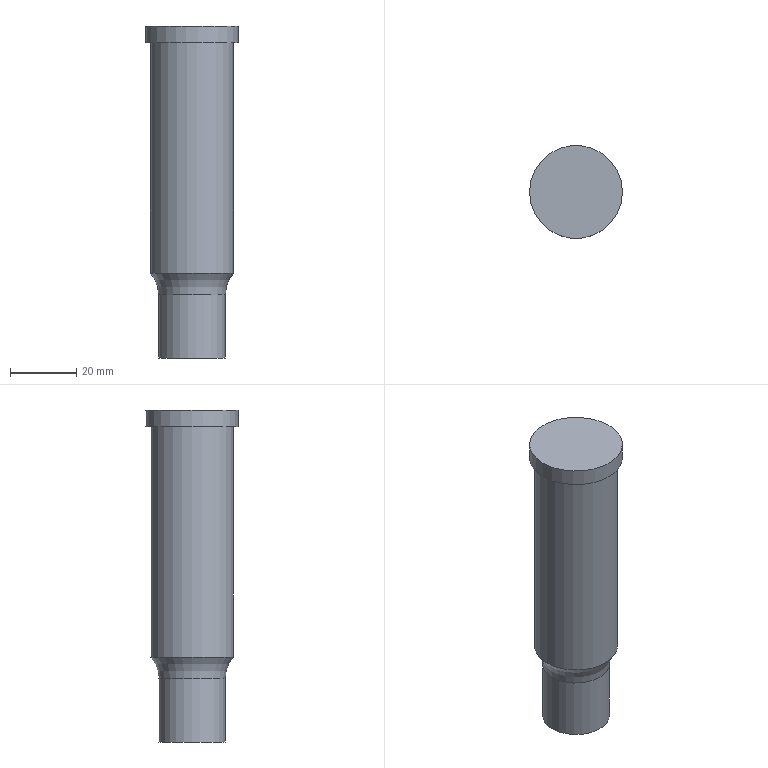Part | NX | features SPAS 25-10-20.10 2 | 1 solid | 7 faces | box 28 x 28 x 100 mm | volume 45618 mm3 | plane 3 | cylinder 3 | torus 1 | commonest cylinder face diameters 20.1 x1 25 x1 28 x1
STEP:
#1=CARTESIAN_POINT('',(-180.846,-11.477,-11.));
#2=VERTEX_POINT('',#1);
#3=CARTESIAN_POINT('',(-190.896,-11.477,-11.));
#4=DIRECTION('',(0.,0.,1.));
#5=DIRECTION('',(1.,0.,0.));
#6=AXIS2_PLACEMENT_3D('',#3,#4,#5);
#7=CIRCLE('',#6,10.05);
#8=EDGE_CURVE('',#2,#2,#7,.T.);
#9=ORIENTED_EDGE('',*,*,#8,.F.);
#10=EDGE_LOOP('',(#9));
#11=FACE_BOUND('',#10,.T.);
#12=CARTESIAN_POINT('',(-190.896,-11.477,-11.));
#13=DIRECTION('',(0.,0.,-1.));
#14=DIRECTION('',(-1.,0.,0.));
#15=AXIS2_PLACEMENT_3D('',#12,#13,#14);
#16=PLANE('',#15);
#17=ADVANCED_FACE('',(#11),#16,.T.);
#18=CARTESIAN_POINT('',(-180.846,-11.477,8.));
#19=VERTEX_POINT('',#18);
#20=CARTESIAN_POINT('',(-190.896,-11.477,8.));
#21=DIRECTION('',(0.,0.,1.));
#22=DIRECTION('',(1.,0.,0.));
#23=AXIS2_PLACEMENT_3D('',#20,#21,#22);
#24=CIRCLE('',#23,10.05);
#25=EDGE_CURVE('',#19,#19,#24,.F.);
#26=ORIENTED_EDGE('',*,*,#25,.T.);
#27=EDGE_LOOP('',(#26));
#28=FACE_BOUND('',#27,.T.);
#29=ORIENTED_EDGE('',*,*,#8,.T.);
#30=EDGE_LOOP('',(#29));
#31=FACE_BOUND('',#30,.T.);
#32=CARTESIAN_POINT('',(-190.896,-11.477,-11.));
#33=DIRECTION('',(0.,0.,1.));
#34=DIRECTION('',(1.,0.,0.));
#35=AXIS2_PLACEMENT_3D('',#32,#33,#34);
#36=CYLINDRICAL_SURFACE('',#35,10.05);
#37=ADVANCED_FACE('',(#28,#31),#36,.T.);
#38=CARTESIAN_POINT('',(-203.396,-11.477,84.));
#39=VERTEX_POINT('',#38);
#40=CARTESIAN_POINT('',(-190.896,-11.477,84.));
#41=DIRECTION('',(0.,0.,-1.));
#42=DIRECTION('',(-1.,0.,0.));
#43=AXIS2_PLACEMENT_3D('',#40,#41,#42);
#44=CIRCLE('',#43,12.5);
#45=EDGE_CURVE('',#39,#39,#44,.F.);
#46=ORIENTED_EDGE('',*,*,#45,.F.);
#47=EDGE_LOOP('',(#46));
#48=FACE_BOUND('',#47,.T.);
#49=CARTESIAN_POINT('',(-178.396,-11.477,14.557));
#50=VERTEX_POINT('',#49);
#51=CARTESIAN_POINT('',(-190.896,-11.477,14.557));
#52=DIRECTION('',(0.,0.,1.));
#53=DIRECTION('',(1.,0.,0.));
#54=AXIS2_PLACEMENT_3D('',#51,#52,#53);
#55=CIRCLE('',#54,12.5);
#56=EDGE_CURVE('',#50,#50,#55,.T.);
#57=ORIENTED_EDGE('',*,*,#56,.T.);
#58=EDGE_LOOP('',(#57));
#59=FACE_BOUND('',#58,.T.);
#60=CARTESIAN_POINT('',(-190.896,-11.477,14.557));
#61=DIRECTION('',(0.,0.,1.));
#62=DIRECTION('',(1.,0.,0.));
#63=AXIS2_PLACEMENT_3D('',#60,#61,#62);
#64=CYLINDRICAL_SURFACE('',#63,12.5);
#65=ADVANCED_FACE('',(#48,#59),#64,.T.);
#66=CARTESIAN_POINT('',(-204.896,-11.477,89.));
#67=VERTEX_POINT('',#66);
#68=CARTESIAN_POINT('',(-190.896,-11.477,89.));
#69=DIRECTION('',(0.,0.,-1.));
#70=DIRECTION('',(-1.,0.,0.));
#71=AXIS2_PLACEMENT_3D('',#68,#69,#70);
#72=CIRCLE('',#71,14.);
#73=EDGE_CURVE('',#67,#67,#72,.T.);
#74=ORIENTED_EDGE('',*,*,#73,.F.);
#75=EDGE_LOOP('',(#74));
#76=FACE_BOUND('',#75,.T.);
#77=CARTESIAN_POINT('',(-190.896,-11.477,89.));
#78=DIRECTION('',(0.,0.,1.));
#79=DIRECTION('',(1.,0.,0.));
#80=AXIS2_PLACEMENT_3D('',#77,#78,#79);
#81=PLANE('',#80);
#82=ADVANCED_FACE('',(#76),#81,.T.);
#83=ORIENTED_EDGE('',*,*,#45,.T.);
#84=EDGE_LOOP('',(#83));
#85=FACE_BOUND('',#84,.T.);
#86=CARTESIAN_POINT('',(-176.896,-11.477,84.));
#87=VERTEX_POINT('',#86);
#88=CARTESIAN_POINT('',(-190.896,-11.477,84.));
#89=DIRECTION('',(0.,0.,1.));
#90=DIRECTION('',(1.,0.,0.));
#91=AXIS2_PLACEMENT_3D('',#88,#89,#90);
#92=CIRCLE('',#91,14.);
#93=EDGE_CURVE('',#87,#87,#92,.T.);
#94=ORIENTED_EDGE('',*,*,#93,.F.);
#95=EDGE_LOOP('',(#94));
#96=FACE_BOUND('',#95,.T.);
#97=CARTESIAN_POINT('',(-190.896,-11.477,84.));
#98=DIRECTION('',(0.,0.,-1.));
#99=DIRECTION('',(-1.,0.,0.));
#100=AXIS2_PLACEMENT_3D('',#97,#98,#99);
#101=PLANE('',#100);
#102=ADVANCED_FACE('',(#85,#96),#101,.T.);
#103=ORIENTED_EDGE('',*,*,#73,.T.);
#104=EDGE_LOOP('',(#103));
#105=FACE_BOUND('',#104,.T.);
#106=ORIENTED_EDGE('',*,*,#93,.T.);
#107=EDGE_LOOP('',(#106));
#108=FACE_BOUND('',#107,.T.);
#109=CARTESIAN_POINT('',(-190.896,-11.477,84.));
#110=DIRECTION('',(0.,0.,1.));
#111=DIRECTION('',(1.,0.,0.));
#112=AXIS2_PLACEMENT_3D('',#109,#110,#111);
#113=CYLINDRICAL_SURFACE('',#112,14.);
#114=ADVANCED_FACE('',(#105,#108),#113,.T.);
#115=ORIENTED_EDGE('',*,*,#25,.F.);
#116=EDGE_LOOP('',(#115));
#117=FACE_BOUND('',#116,.T.);
#118=ORIENTED_EDGE('',*,*,#56,.F.);
#119=EDGE_LOOP('',(#118));
#120=FACE_BOUND('',#119,.T.);
#121=CARTESIAN_POINT('',(-190.896,-11.477,8.));
#122=DIRECTION('',(0.,0.,1.));
#123=DIRECTION('',(1.,0.,0.));
#124=AXIS2_PLACEMENT_3D('',#121,#122,#123);
#125=TOROIDAL_SURFACE('',#124,20.05,10.);
#126=ADVANCED_FACE('',(#117,#120),#125,.F.);
#127=CLOSED_SHELL('',(#17,#37,#65,#82,#102,#114,#126));
#128=MANIFOLD_SOLID_BREP('',#127);
#129=(LENGTH_UNIT()NAMED_UNIT(*)SI_UNIT(.MILLI.,.METRE.));
#130=UNCERTAINTY_MEASURE_WITH_UNIT(LENGTH_MEASURE(0.00001),#129,'','');
#131=(NAMED_UNIT(*)PLANE_ANGLE_UNIT()SI_UNIT($,.RADIAN.));
#132=(NAMED_UNIT(*)SI_UNIT($,.STERADIAN.)SOLID_ANGLE_UNIT());
#133=(GEOMETRIC_REPRESENTATION_CONTEXT(3)GLOBAL_UNCERTAINTY_ASSIGNED_CONTEXT((#130))GLOBAL_UNIT_ASSIGNED_CONTEXT((#129,#131,#132))REPRESENTATION_CONTEXT('',''));
#134=ADVANCED_BREP_SHAPE_REPRESENTATION('',(#128),#133);